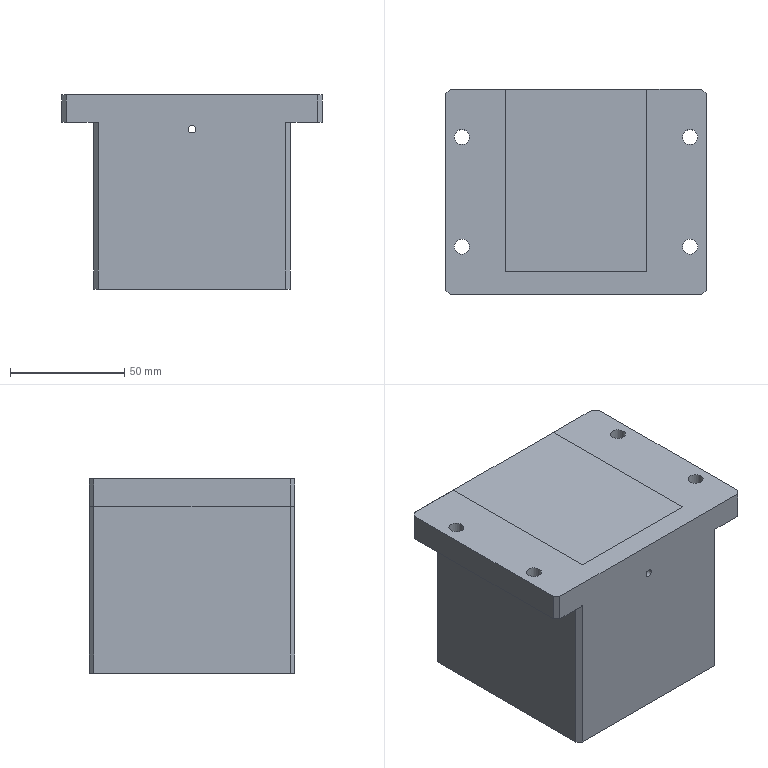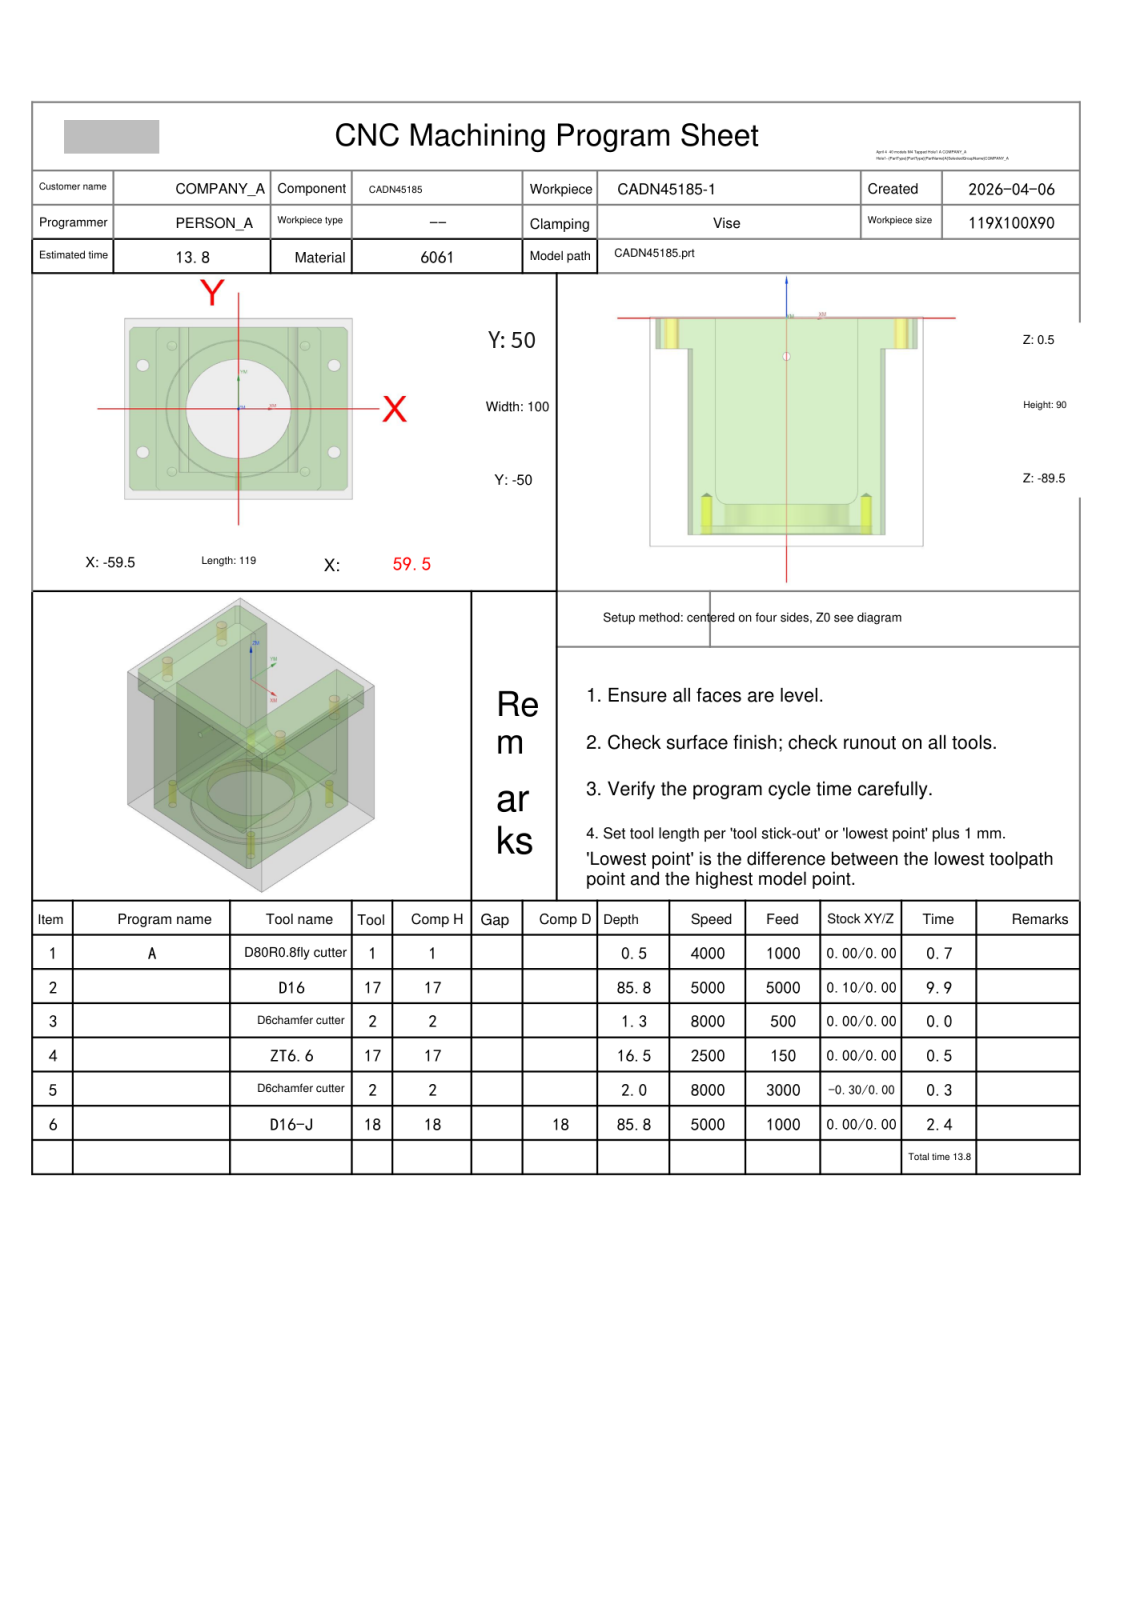NC program | NX | posted by the shop | part box 114 x 90 x 85 mm
Lines 1 to 34 of 2085:
%
O0001
(Machine time: 14.96 MIN)
(===Total Tool:4===)
(T1=D80R0.8飞刀 D=80.  R=0.8  D-  H01 Z=0.    )
(T17=D16    D=16.  R=0.   D-  H17 Z=-85.3 )
(T2=D6chamfer cutter   D=6.   R=0.   D-  H02 Z=-1.5  )
(T18=D16-J  D=16.  R=0.   D18 H18 Z=-85.3 )
G80 G90 G17 G49 G40
G91 G28 Z0
M01
N1 T01 M06
(D80R0.8飞刀  D=80. R=0.8 H=01 ce=0.00 di=0.00)
G00 G90 G54 X-102. Y42.5 M03 S4000
G43 H01 Z20.
M08
Z2.
G01 Z0.0 F1000.
X-97.
X97.
Y0.0
X-97.
Y-42.5
X97.
X102.
Z2.
G00 Z20.
G91 G28 Z0.0
M05
M09
G91 G28 Z0.0
M01